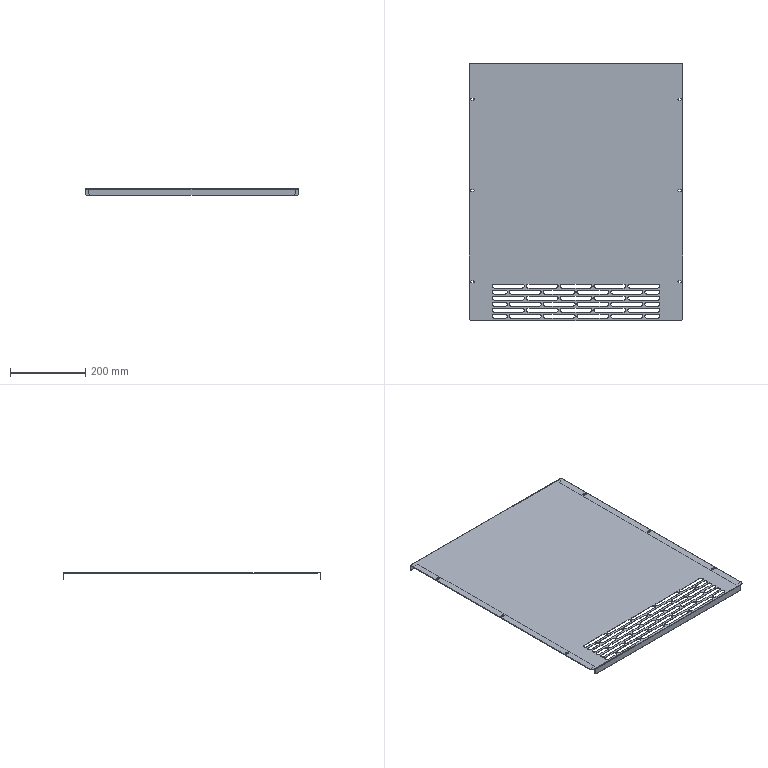Part | STEP file | HESS-408-70-15W-N-15-inner liner closing plate | 1 solid | 275 faces | box 568 x 685 x 18 mm | volume 406764 mm3 | cylinder 149 | plane 126 | commonest cylinder face diameters 10 x103 5 x18 6 x18 0.1 x4 2.1 x4 20 x2